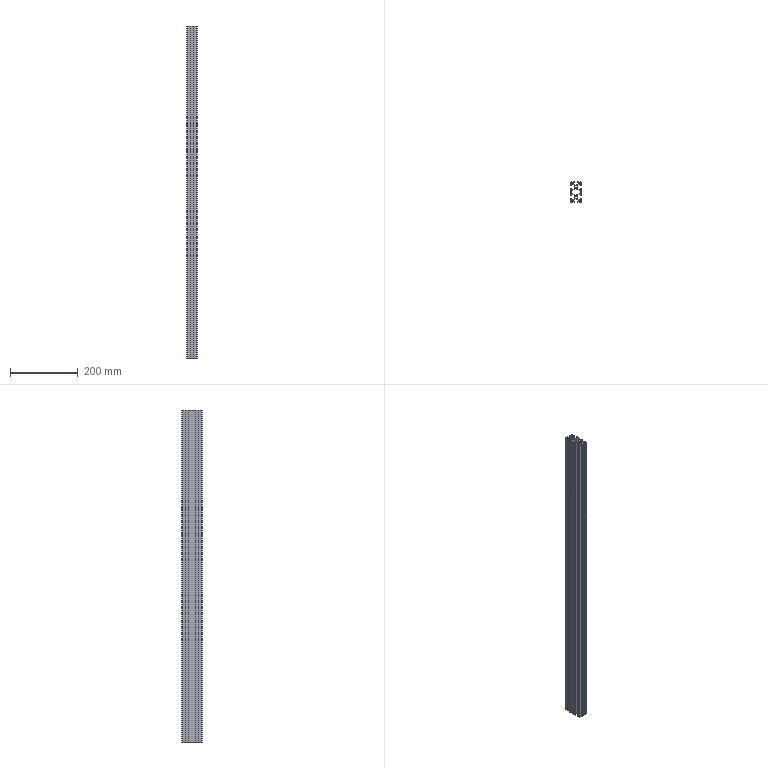Part | SolidWorks | features WeldMemberFeat 1, WeldmentFeature 1 | 1 solid | 126 faces | box 30 x 60 x 980 mm | volume 490298 mm3 | plane 118 | cylinder 8 | commonest cylinder face diameters 9.2 x4 3 x2 5 x2